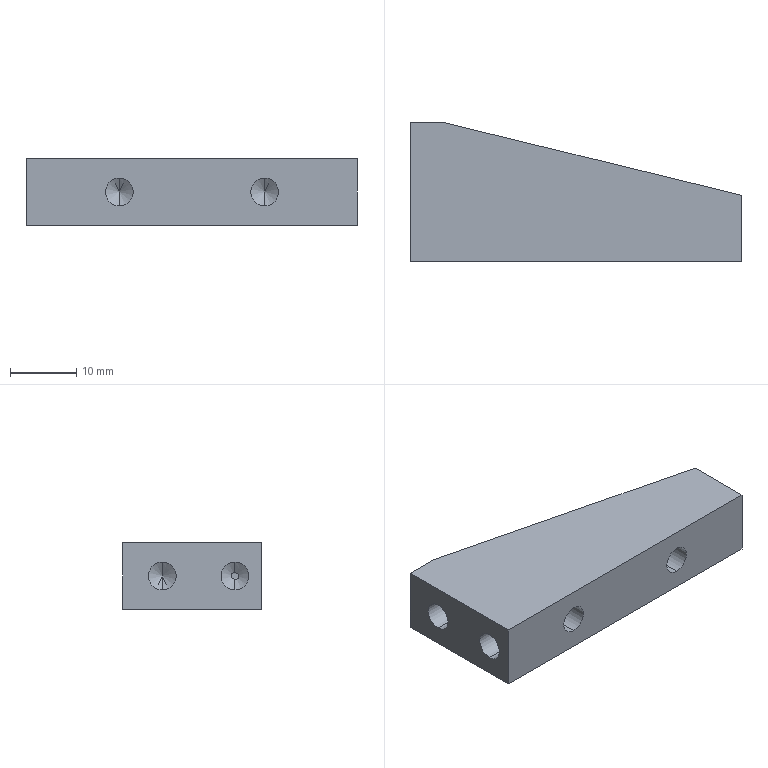Part | STEP file | reinforcing plate 5 | 1 solid | 23 faces | box 50 x 21 x 10 mm | volume 7392 mm3 | cylinder 8 | cone 8 | plane 7 | commonest cylinder face diameters 4.2 x8